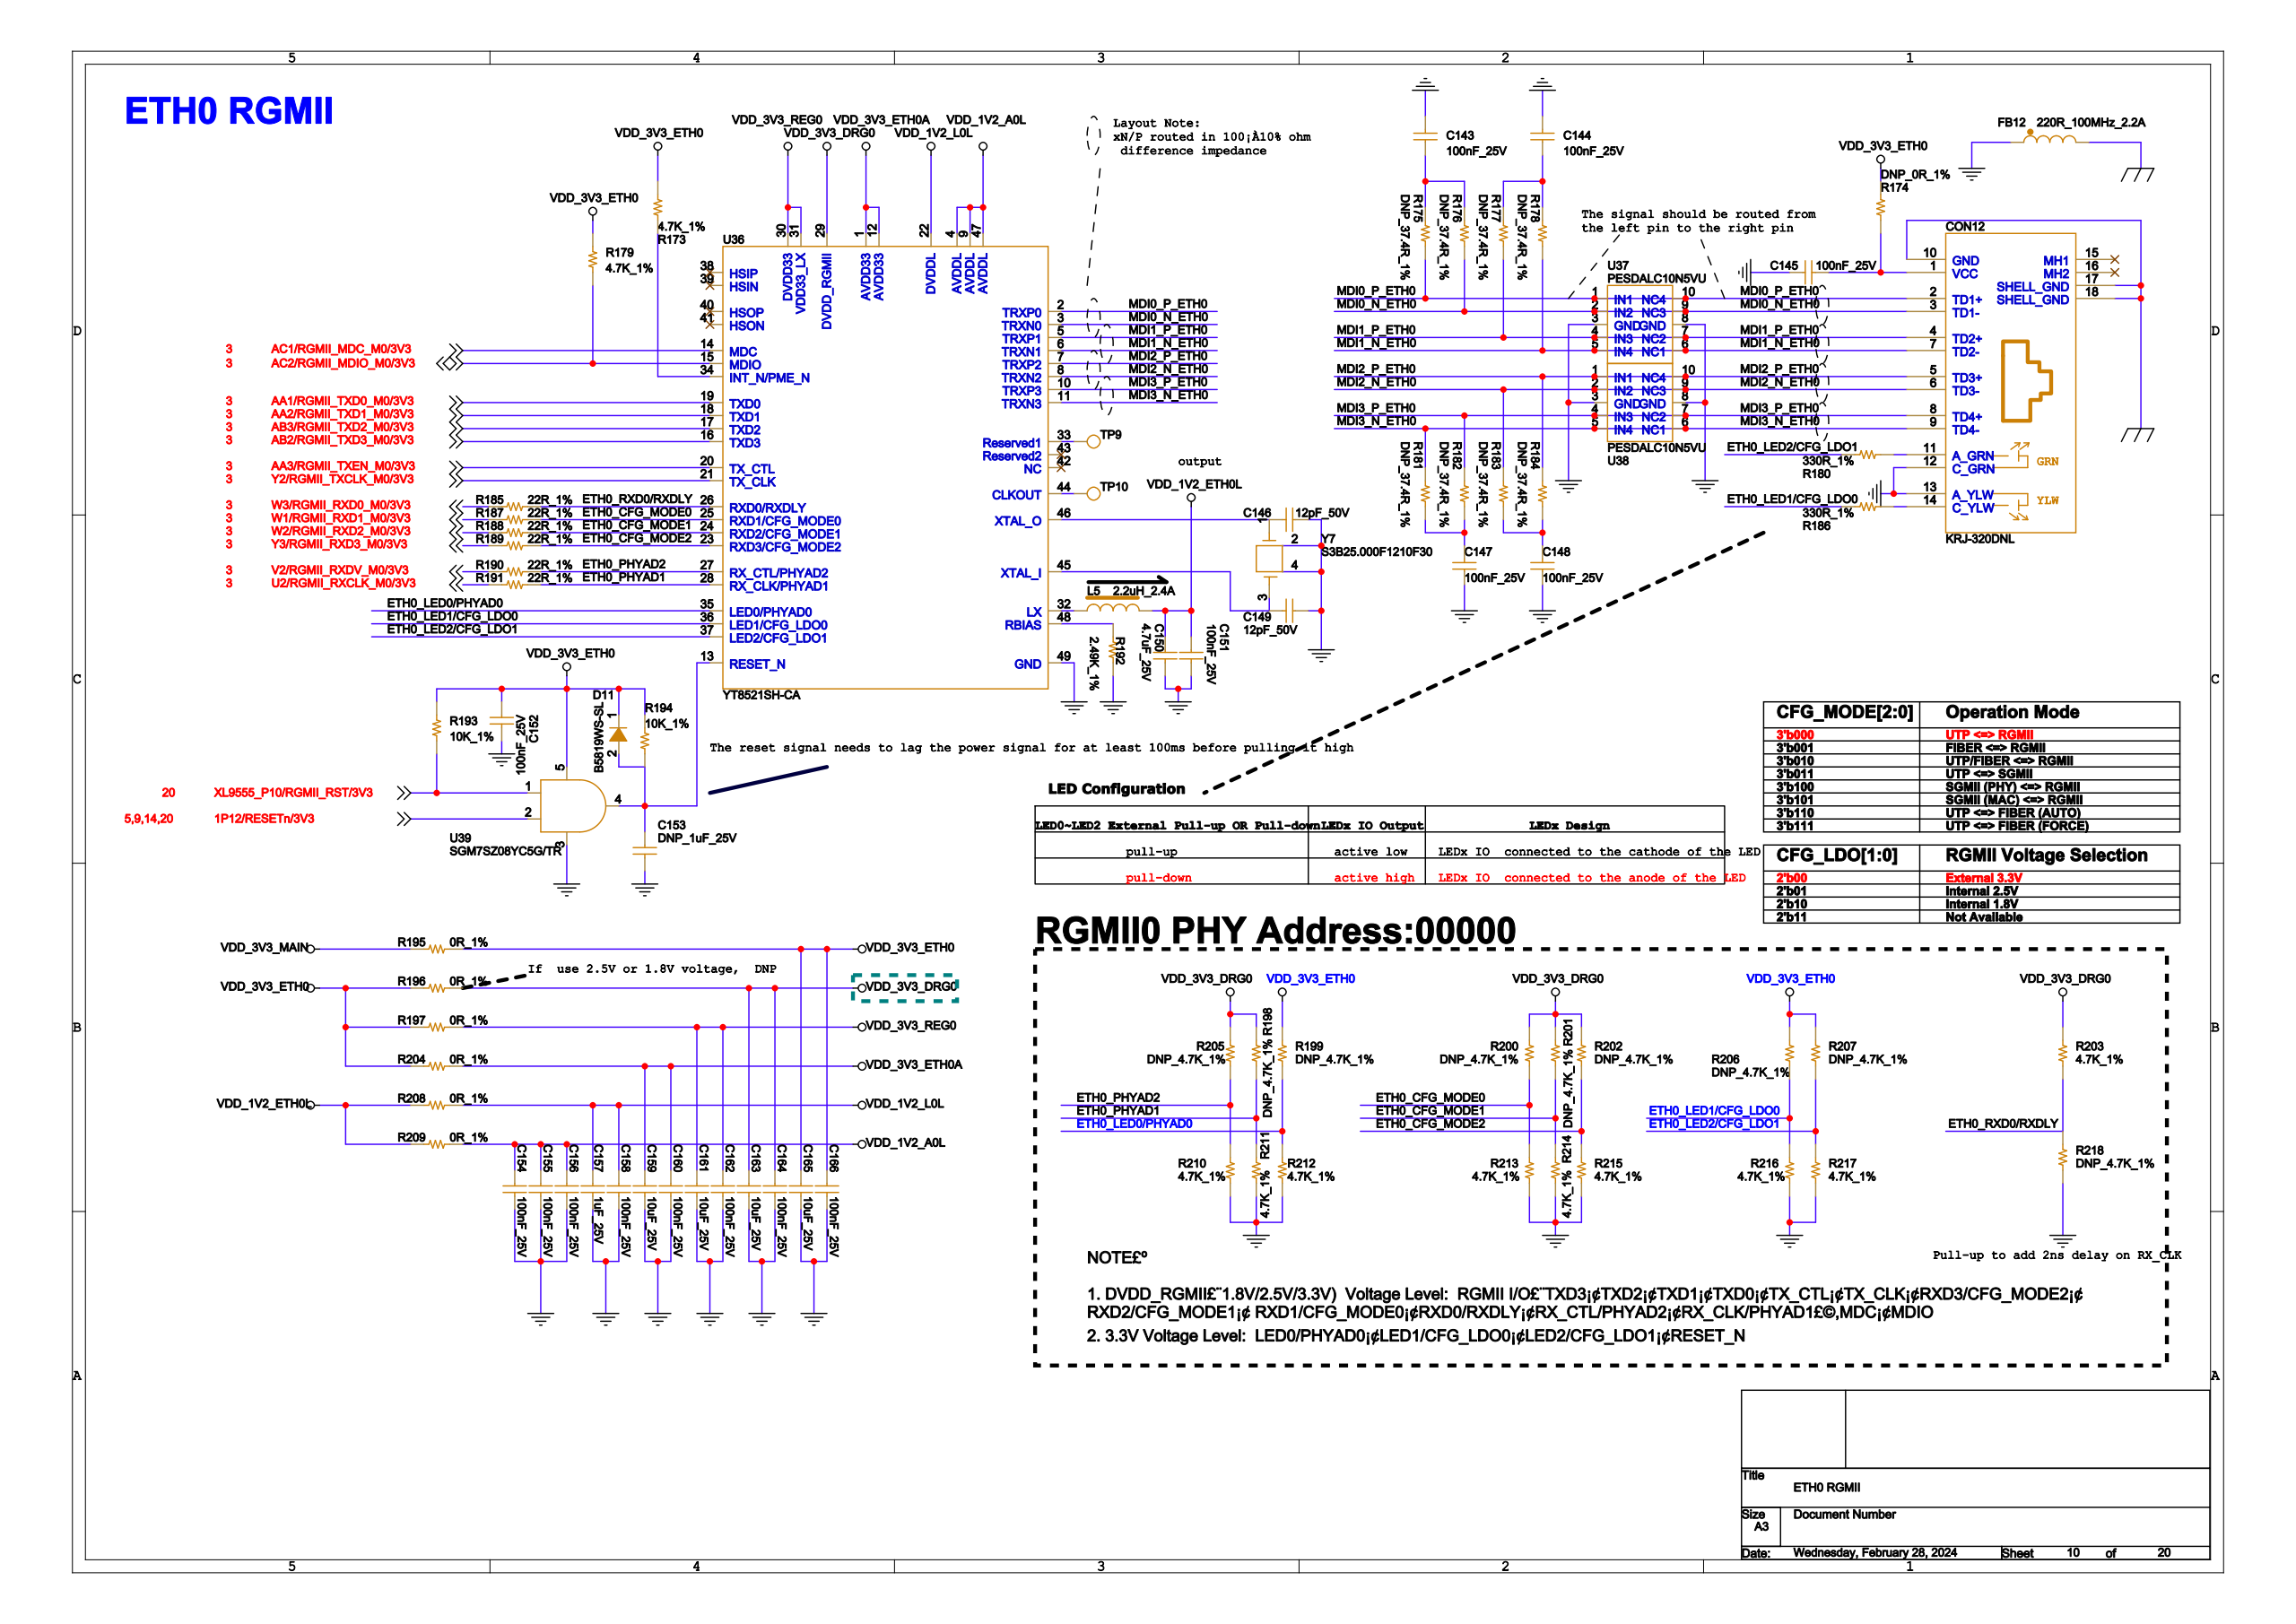Circuit board | Cadence Allegro | 1024 parts | 682 nets | one sheet of the schematic
Parts on this sheet (reference | value | footprint):
C143 | 100nF_25V | C0402
C144 | 100nF_25V | C0402
C145 | 100nF_25V | C0402
C146 | 12pF_50V | C0402
C147 | 100nF_25V | C0402
C148 | 100nF_25V | C0402
C149 | 12pF_50V | C0402
C150 | 4.7uF_25V | C0603
C151 | 100nF_25V | C0402
C152 | 100nF_25V | C0402
C153 | DNP_1uF_25V | C0603
C154 | 100nF_25V | C0402
C155 | 100nF_25V | C0402
C156 | 100nF_25V | C0402
C157 | 1uF_25V | C0603
C158 | 100nF_25V | C0402
C159 | 10uF_25V | C0603
C160 | 100nF_25V | C0402
C161 | 10uF_25V | C0603
C162 | 100nF_25V | C0402
C163 | 10uF_25V | C0603
C164 | 100nF_25V | C0402
C165 | 10uF_25V | C0603
C166 | 100nF_25V | C0402
CON12 | KRJ-320DNL | KRJ-320DNL_14P
FB12 | 220R_100MHz_2A | L0603
L5 | 2.2uH_2.4A | SMD-L2520M-2P
R173 | 4.7K_1% | R0402
R174 | DNP_0R_1% | R0402
R175 | DNP_37.4R_1% | R0603
R176 | DNP_37.4R_1% | R0603
R177 | DNP_37.4R_1% | R0603
R178 | DNP_37.4R_1% | R0603
R179 | 4.7K_1% | R0402
R180 | 330R_1% | R0402
R181 | DNP_37.4R_1% | R0603
R182 | DNP_37.4R_1% | R0603
R183 | DNP_37.4R_1% | R0603
R184 | DNP_37.4R_1% | R0603
R185 | 22R_1% | R0402
R186 | 330R_1% | R0402
R187 | 22R_1% | R0402
R188 | 22R_1% | R0402
R189 | 22R_1% | R0402
R190 | 22R_1% | R0402
R191 | 22R_1% | R0402
R192 | 2.49K_1% | R0603
R193 | 10K_1% | R0402
R194 | 10K_1% | R0402
R195 | 0R_1% | R0603
R196 | 0R_1% | R0603
R197 | 0R_1% | R0603
R198 | DNP_4.7K_1% | R0402
R199 | DNP_4.7K_1% | R0402
R200 | DNP_4.7K_1% | R0402
R201 | DNP_4.7K_1% | R0402
R202 | DNP_4.7K_1% | R0402
R203 | 4.7K_1% | R0402
R204 | 0R_1% | R0603
R205 | DNP_4.7K_1% | R0402
R206 | DNP_4.7K_1% | R0402
R207 | DNP_4.7K_1% | R0402
R208 | 0R_1% | R0603
R209 | 0R_1% | R0603
R210 | 4.7K_1% | R0402
R211 | 4.7K_1% | R0402
R212 | 4.7K_1% | R0402
R213 | 4.7K_1% | R0402
R214 | 4.7K_1% | R0402
R215 | 4.7K_1% | R0402
R216 | 4.7K_1% | R0402
R217 | 4.7K_1% | R0402
R218 | DNP_4.7K_1% | R0402
TP9 | SMT TP | TP30
TP10 | SMT TP | TP30
U36 | YT8521SH-CA | QFN48
U37 | PESDALC10N5VU | DFN-10-2510
U38 | PESDALC10N5VU | DFN-10-2510
U39 | SGM7SZ08YC5G/TR | SC70-5-43M
Y7 | S3B25.000F1210F30 | SMD_3225
Nets of these parts (net: part-pin ...):
GND: C143-2 C144-2 C145-1 C146-1 C147-1 C148-1 C149-1 C150-2 C151-2 C152-2 C153-2 C154-2 C155-2 C156-2 C157-2 C158-2 C159-2 C160-2 C161-2 C162-2 C163-2 C164-2 C165-2 C166-2 CON12-12 CON12-13 FB12-1 R192-1 R210-1 R211-1 R212-1 R213-1 R214-1 R215-1 R216-1 R217-1 R218-1 U37-3 U37-8 U38-3 U38-8 U39-3 Y7-2 Y7-4 U36-49
EGND: CON12-10 CON12-17 CON12-18 FB12-2
VDD_3V3_MAIN: R195-1
1P12/RESETN/3V3: U39-2
N21604673: C146-2 Y7-1 U36-46
N21604675: C149-2 Y7-3 U36-45
VDD_1V2_ETH0L: C150-1 C151-1 L5-2 R208-1 R209-1
Y2/RGMII_TXCLK_M0/3V3: U36-21
Y3/RGMII_RXD3_M0/3V3: R189-1
V2/RGMII_RXDV_M0/3V3: R190-1
U2/RGMII_RXCLK_M0/3V3: R191-1
AA3/RGMII_TXEN_M0/3V3: U36-20
AB2/RGMII_TXD3_M0/3V3: U36-16
AB3/RGMII_TXD2_M0/3V3: U36-17
AA2/RGMII_TXD1_M0/3V3: U36-18
AA1/RGMII_TXD0_M0/3V3: U36-19
W3/RGMII_RXD0_M0/3V3: R185-1
W2/RGMII_RXD2_M0/3V3: R188-1
W1/RGMII_RXD1_M0/3V3: R187-1
N21604532: CON12-11 R180-2
N21604655: CON12-14 R186-2
MDI0_P_ETH0: CON12-2 R175-2 U37-1 U37-10 U36-2
MDI0_N_ETH0: CON12-3 R176-2 U37-2 U37-9 U36-3
MDI1_P_ETH0: CON12-4 R177-2 U37-4 U37-7 U36-5
MDI1_N_ETH0: CON12-7 R178-2 U37-5 U37-6 U36-6
MDI2_P_ETH0: CON12-5 R184-1 U38-1 U38-10 U36-7
MDI2_N_ETH0: CON12-6 R183-1 U38-2 U38-9 U36-8
MDI3_P_ETH0: CON12-8 R182-1 U38-4 U38-7 U36-10
MDI3_N_ETH0: CON12-9 R181-1 U38-5 U38-6 U36-11
N21604537: C145-2 CON12-1 R174-2
N21603124: C153-1 R194-1 U39-4 U36-13
VDD_3V3_ETH0: C152-1 C165-1 C166-1 R173-2 R174-1 R179-1 R193-1 R194-2 R195-2 R196-1 R197-1 R199-2 R204-1 R206-2 R207-2 U39-5
N21604256: L5-1 U36-32
VDD_3V3_DRG0: C163-1 C164-1 R196-2 R198-2 R200-2 R201-2 R202-2 R203-2 R205-2 U36-29
VDD_3V3_REG0: C161-1 C162-1 R197-2 U36-30 U36-31
VDD_3V3_ETH0A: C159-1 C160-1 R204-2 U36-1 U36-12
VDD_1V2_L0L: C157-1 C158-1 R208-2 U36-22
VDD_1V2_A0L: C154-1 C155-1 C156-1 R209-2 U36-4 U36-9 U36-47
N21604710: R173-1 U36-34
AC2/RGMII_MDIO_M0/3V3: R179-2 U36-15
ETH0_RXD0/RXDLY: R185-2 R203-1 R218-2 U36-26
ETH0_PHYAD2: R190-2 R205-1 R210-2 U36-27
ETH0_PHYAD1: R191-2 R198-1 R211-2 U36-28
ETH0_LED0/PHYAD0: R199-1 R212-2 U36-35
ETH0_CFG_MODE0: R187-2 R200-1 R213-2 U36-25
ETH0_CFG_MODE1: R188-2 R201-1 R214-2 U36-24
ETH0_CFG_MODE2: R189-2 R202-1 R215-2 U36-23
ETH0_LED1/CFG_LDO0: R186-1 R206-1 R216-2 U36-36
ETH0_LED2/CFG_LDO1: R180-1 R207-1 R217-2 U36-37
N21604240: R192-2 U36-48
N21604226: TP10-1 U36-44
N21604228: TP9-1 U36-33
XL9555_P10/RGMII_RST/3V3: R193-2 U39-1
AC1/RGMII_MDC_M0/3V3: U36-14
N21604562: C143-1 R175-1 R176-1
N21604570: C144-1 R177-1 R178-1
N21604574: C147-2 R181-2 R182-2
N21604582: C148-2 R183-2 R184-2